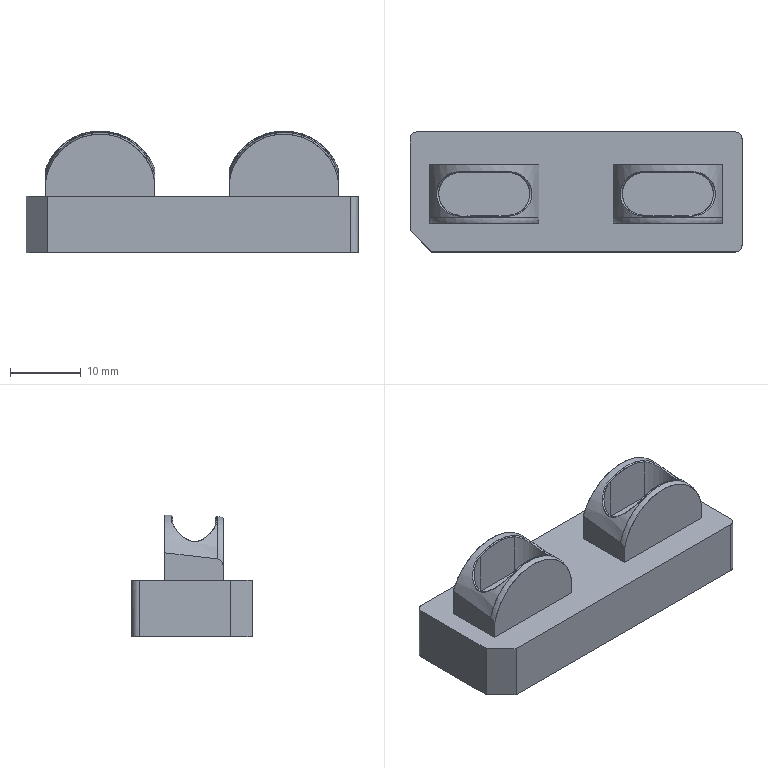NC program | PowerMill | posted with a generic post | part box 47 x 17 x 17.251 mm
Lines 18301 to 19119 of 158620:
N18398 M6
N18399 S8500 M03
N18400 G00 G90 X0.0 Y0.0
N18401 G43 Z9.8013 H3
N18402
N18403 G05 P10000 R8
N18404 X-25.6664 Y-17.9294
N18405 Z-8.25
N18406 G01 Z-9.45 F360.0
N18407 X-23.1365 Y-13.3007 F600.0
N18408 X-16.1394 Y-9.8021
N18409 X-20.3885
N18410 X-20.9549 Y-9.7974
N18411 G02 X-21.5212 Y-9.7435 I0.3338 J6.5029
N18412 G02 X-22.0876 Y-9.6275 I0.9782 J6.2202
N18413 G01 X-22.3708 Y-9.5453
N18414 G02 X-22.8859 Y-9.3503 I1.9528 J5.9372
N18415 G01 X-23.2203 Y-9.1901
N18416 X-23.5035 Y-9.0309
N18417 X-23.8008 Y-8.8385
N18418 X-24.1154 Y-8.6019
N18419 X-24.353 Y-8.3976
N18420 X-24.5418 Y-8.2169
N18421 X-24.7406 Y-8.0061
N18422 X-24.8895 Y-7.8308
N18423 X-25.0319 Y-7.6502
N18424 X-25.2306 Y-7.3669
N18425 X-25.4038 Y-7.0835
N18426 X-25.4857 Y-6.9339
N18427 X-25.5885 Y-6.7272
N18428 X-25.6837 Y-6.5169
N18429 X-25.794 Y-6.2335
N18430 X-25.8533 Y-6.0545
N18431 X-25.907 Y-5.8737
N18432 X-25.9622 Y-5.6668
N18433 X-26.0115 Y-5.4325
N18434 X-26.052 Y-5.1964
N18435 X-26.0938 Y-4.8168
N18436 X-26.1059 Y-4.5336
N18437 X-26.1081 Y3.6835
N18438 G02 X-26.0938 Y4.2501 I7.9765 J0.0813
N18439 G01 X-26.052 Y4.63
N18440 X-26.0216 Y4.8168
N18441 X-25.9622 Y5.1001
N18442 X-25.8867 Y5.3835
N18443 X-25.7943 Y5.6668
N18444 X-25.6837 Y5.9502
N18445 G02 X-25.4038 Y6.5169 I5.3267 J-2.2781
N18446 G01 X-25.2308 Y6.8002
N18447 X-25.0322 Y7.0835
N18448 X-24.9193 Y7.2288
N18449 X-24.7406 Y7.4395
N18450 X-24.5421 Y7.6502
N18451 X-24.353 Y7.8312
N18452 X-24.1157 Y8.0352
N18453 X-23.9528 Y8.1606
N18454 X-23.7866 Y8.2817
N18455 X-23.5035 Y8.4647
N18456 X-23.2203 Y8.6237
N18457 X-22.8868 Y8.7836
N18458 X-22.6539 Y8.8793
N18459 X-22.3708 Y8.9788
N18460 X-22.0876 Y9.0611
N18461 G02 X-21.5212 Y9.1771 I1.6038 J-6.3927
N18462 G02 X-20.9549 Y9.231 I0.8987 J-6.4341
N18463 G01 X-20.3885 Y9.2357
N18464 X-5.6635
N18465 X-5.0971 Y9.233
N18466 G02 X-4.5308 Y9.1845 I-0.264 J-6.4244
N18467 G02 X-3.9644 Y9.0744 I-0.9261 J-6.2735
N18468 G01 X-3.7406 Y9.0118
N18469 X-3.3981 Y8.899
N18470 X-3.1133 Y8.7836
N18471 X-2.8318 Y8.6505
N18472 X-2.5486 Y8.4955
N18473 X-2.2654 Y8.3174
N18474 X-2.1216 Y8.2169
N18475 X-1.9103 Y8.0562
N18476 X-1.699 Y7.878
N18477 X-1.4579 Y7.6502
N18478 G02 X-0.9679 Y7.0835 I-4.0616 J-4.0072
N18479 G01 X-0.8187 Y6.8709
N18480 G03 X0.8189 Y6.871 I0.8187 J0.5741
N18481 G01 X0.9679 Y7.0835
N18482 G02 X1.288 Y7.4714 I4.8718 J-3.6948
N18483 G01 X1.4579 Y7.6502
N18484 X1.699 Y7.878
N18485 X1.9103 Y8.0562
N18486 X2.0856 Y8.1898
N18487 X2.2654 Y8.3174
N18488 X2.5486 Y8.4955
N18489 X2.875 Y8.671
N18490 X3.1133 Y8.7836
N18491 X3.3981 Y8.899
N18492 X3.6813 Y8.9952
N18493 G02 X4.2476 Y9.1375 I1.8784 J-6.2784
N18494 G02 X4.814 Y9.2163 I1.1555 J-6.2283
N18495 G01 X5.0971 Y9.233
N18496 X5.6635 Y9.2357
N18497 X20.3885
N18498 X20.9549 Y9.231
N18499 G02 X21.5212 Y9.1771 I-0.3381 J-6.5471
N18500 G02 X22.0876 Y9.0611 I-1.0072 J-6.3617
N18501 G01 X22.2767 Y9.007
N18502 X22.6539 Y8.8793
N18503 X22.8868 Y8.7836
N18504 X23.2203 Y8.6237
N18505 X23.5035 Y8.4647
N18506 X23.6926 Y8.3433
N18507 X23.8784 Y8.2169
N18508 X24.1157 Y8.0352
N18509 X24.353 Y7.8312
N18510 X24.5421 Y7.6502
N18511 X24.7409 Y7.4395
N18512 X24.8896 Y7.2641
N18513 X25.0322 Y7.0836
N18514 X25.2308 Y6.8002
N18515 X25.3408 Y6.622
N18516 X25.4857 Y6.3677
N18517 X25.5903 Y6.159
N18518 X25.6662 Y5.9898
N18519 X25.7942 Y5.6668
N18520 X25.8867 Y5.3835
N18521 X25.9623 Y5.1002
N18522 X26.0216 Y4.8168
N18523 X26.052 Y4.63
N18524 X26.0938 Y4.2501
N18525 X26.1072 Y3.9668
N18526 Y-4.5335
N18527 X26.0938 Y-4.8168
N18528 X26.052 Y-5.1964
N18529 X26.0117 Y-5.4325
N18530 X25.9623 Y-5.6668
N18531 X25.8866 Y-5.9502
N18532 X25.7942 Y-6.2335
N18533 X25.6837 Y-6.5169
N18534 X25.5903 Y-6.7254
N18535 X25.4857 Y-6.9339
N18536 X25.4038 Y-7.0835
N18537 X25.2308 Y-7.3669
N18538 X25.0104 Y-7.6787
N18539 X24.9193 Y-7.7952
N18540 X24.7405 Y-8.0061
N18541 X24.5419 Y-8.2169
N18542 X24.353 Y-8.3976
N18543 X24.1154 Y-8.6019
N18544 X23.8163 Y-8.8277
N18545 X23.5035 Y-9.0309
N18546 X23.2203 Y-9.1901
N18547 X22.8859 Y-9.3503
N18548 X22.7006 Y-9.4269
N18549 X22.3708 Y-9.5453
N18550 G02 X21.8044 Y-9.6934 I-1.8826 J6.0394
N18551 G02 X21.2381 Y-9.7779 I-1.2236 J6.2663
N18552 G01 X20.9549 Y-9.7974
N18553 X20.3885 Y-9.8021
N18554 X5.6635
N18555 X5.0971 Y-9.7994
N18556 G02 X4.5308 Y-9.7509 I0.2749 J6.5522
N18557 G01 X4.3361 Y-9.7192
N18558 X3.9644 Y-9.6408
N18559 X3.6813 Y-9.5616
N18560 X3.3709 Y-9.4544
N18561 X3.1138 Y-9.3503
N18562 X2.8317 Y-9.2169
N18563 X2.5486 Y-9.0618
N18564 X2.2654 Y-8.8838
N18565 X2.0858 Y-8.7562
N18566 X1.9106 Y-8.6228
N18567 X1.699 Y-8.4444
N18568 X1.4582 Y-8.2169
N18569 X1.288 Y-8.0379
N18570 X1.101 Y-7.8187
N18571 X0.9679 Y-7.6502
N18572 X0.8189 Y-7.4377
N18573 G03 X-0.8187 Y-7.4375 I-0.8189 J-0.574
N18574 G01 X-0.9485 Y-7.6226
N18575 X-1.1327 Y-7.8589
N18576 X-1.2917 Y-8.0412
N18577 X-1.4582 Y-8.2169
N18578 X-1.7382 Y-8.4774
N18579 X-1.9106 Y-8.6228
N18580 X-2.0859 Y-8.7561
N18581 X-2.2654 Y-8.8838
N18582 X-2.5486 Y-9.0619
N18583 X-2.8317 Y-9.2169
N18584 X-3.1138 Y-9.3503
N18585 X-3.3981 Y-9.4654
N18586 X-3.6813 Y-9.5616
N18587 X-3.9644 Y-9.6408
N18588 X-4.1458 Y-9.6818
N18589 X-4.3282 Y-9.7172
N18590 X-4.5308 Y-9.7509
N18591 X-4.814 Y-9.7825
N18592 X-5.0971 Y-9.7994
N18593 X-5.6635 Y-9.8021
N18594 X-16.1394
N18595 G00 Z9.8013
N18596 G05 P0
N18597 (---------------)
N18598 ( END TOOLPATH : 精公基准台01-基准面偏置-D10 )
N18599 (---------------)
N18600 ( START TOOLPATH : 精公基准台01-外形侧光-D10 )
N18601 (---------------)
N18602 G00 X0.0 Y0.0 Z10.798
N18603 G05 P10000 R8
N18604 X-1.0177 Y-7.9884
N18605 Z-8.22
N18606 G01 Z-9.42 F360.0
N18607 G03 X-2.1184 Y-8.3147 I-0.1564 J-1.4919 F600.0
N18608 G02 X-5.2941 Y-9.432 I-3.1541 J3.8933
N18609 G01 X-12.9615 Y-9.4317
N18610 X-20.8143 Y-9.4313
N18611 G02 X-25.738 Y-4.3814 I0.0867 J5.0098
N18612 G01 Y3.8348
N18613 G02 X-20.8114 Y8.8649 I5.0101 J0.0207
N18614 G01 X-5.293 Y8.8656
N18615 G02 X-0.262 Y3.8337 I0.0208 J-5.0102
N18616 G01 Y-0.2846
N18617 Y-4.3822
N18618 G02 X-2.1184 Y-8.3147 I-5.0105 J-0.0392
N18619 G03 X-2.6659 Y-9.3238 I0.9443 J-1.1656
N18620 G01 X-1.0827 Y-7.9439
N18621 G03 X-2.1848 Y-8.2656 I-0.1627 J-1.4911
N18622 G02 X-5.2941 Y-9.352 I-3.0877 J3.8442
N18623 G01 X-12.9615
N18624 X-20.6289
N18625 G02 X-25.658 Y-4.3814 I-0.0957 J4.9326
N18626 G01 Y3.8337
N18627 G02 X-20.6289 Y8.7857 I4.933 J0.0198
N18628 G01 X-5.2941
N18629 G02 X-0.342 Y3.8337 I0.0219 J-4.9303
N18630 G01 Y-0.2846
N18631 Y-4.3814
N18632 G02 X-2.1848 Y-8.2656 I-4.9305 J-0.04
N18633 G03 X-2.7366 Y-9.2723 I0.9394 J-1.1694
N18634 G00 Z4.0618
N18635 G01 X24.9817 Y-7.9893 F10000.0
N18636 G00 Z-8.22
N18637 G01 Z-9.42 F360.0
N18638 G03 X23.8809 Y-8.3154 I-0.1568 J-1.4918 F600.0
N18639 G02 X20.8114 Y-9.4313 I-3.1532 J3.8939
N18640 G01 X5.293 Y-9.432
N18641 G02 X0.4219 Y-5.6778 I-0.0208 J5.0102
N18642 G02 X0.262 Y-4.3814 I4.8652 J1.2583
N18643 G01 Y-0.2846
N18644 Y3.8348
N18645 G02 X5.2941 Y8.8657 I5.0103 J0.0206
N18646 G01 X20.8143 Y8.8649
N18647 G02 X25.738 Y3.8337 I-0.0864 J-5.0095
N18648 G01 Y-4.3822
N18649 G02 X23.8809 Y-8.3154 I-5.0103 J-0.0393
N18650 G03 X23.3331 Y-9.3243 I0.944 J-1.1657
N18651 G01 X24.9156 Y-7.9449
N18652 G03 X23.8135 Y-8.2663 I-0.163 J-1.4911
N18653 G02 X20.6289 Y-9.352 I-3.0889 J3.8469
N18654 G01 X5.2941
N18655 G02 X0.4997 Y-5.6592 I-0.0219 J4.9302
N18656 G02 X0.342 Y-4.3814 I4.7864 J1.2396
N18657 G01 Y-0.2846
N18658 Y3.8337
N18659 G02 X5.2941 Y8.7857 I4.9302 J0.0217
N18660 G01 X20.6289
N18661 G02 X25.658 Y3.8337 I0.096 J-4.9322
N18662 G01 Y-4.3814
N18663 G02 X23.8135 Y-8.2663 I-4.9334 J-0.038
N18664 G03 X23.2615 Y-9.273 I0.9391 J-1.1697
N18665 G00 Z10.798
N18666 G05 P0
N18667 (---------------)
N18668 ( END TOOLPATH : 精公基准台01-外形侧光-D10 )
N18669 (---------------)
N18670 ( START TOOLPATH : 精公基准台01-基准台侧光-D10 )
N18671 (---------------)
N18672 G00 X0.0 Y0.0 Z9.8013
N18673 G05 P10000 R8
N18674 X28.7413 Y-16.6514
N18675 Z-16.15
N18676 G01 Z-17.35 F360.0
N18677 G03 X25.8898 Y-12.5442 I-1.4257 J2.0536 F600.0
N18678 G01 X25.8115 Y-12.5985
N18679 X25.8099 Y-12.5996
N18680 X25.8083 Y-12.6006
N18681 X25.6279 Y-12.7136
N18682 X25.6268 Y-12.7143
N18683 X25.6257 Y-12.715
N18684 X25.49 Y-12.7939
N18685 X25.4885 Y-12.7948
N18686 X25.487 Y-12.7956
N18687 X25.1708 Y-12.9619
N18688 X25.1693 Y-12.9627
N18689 X25.1677 Y-12.9635
N18690 X25.0174 Y-13.0343
N18691 X25.0164 Y-13.0348
N18692 X25.0153 Y-13.0353
N18693 X24.8494 Y-13.1077
N18694 X24.8478 Y-13.1084
N18695 X24.8462 Y-13.109
N18696 X24.5301 Y-13.231
N18697 X24.5278 Y-13.2319
N18698 X24.5254 Y-13.2326
N18699 X24.1404 Y-13.3544
N18700 X24.1384 Y-13.355
N18701 X24.1363 Y-13.3556
N18702 X23.8889 Y-13.4192
N18703 X23.887 Y-13.4197
N18704 X23.885 Y-13.4201
N18705 X23.5688 Y-13.4846
N18706 X23.5669 Y-13.485
N18707 X23.5649 Y-13.4853
N18708 X23.2488 Y-13.5337
N18709 X23.2465 Y-13.534
N18710 X23.2443 Y-13.5342
N18711 X22.9281 Y-13.5642
N18712 X22.9262 Y-13.5644
N18713 X22.9242 Y-13.5645
N18714 X22.608 Y-13.5788
N18715 X22.6064 Y-13.5789
N18716 X22.6047
N18717 X22.2885 Y-13.58
N18718 X22.2884
N18719 X22.2883
N18720 X-20.3914
N18721 X-20.3919
N18722 X-20.3925
N18723 X-20.7086 Y-13.5757
N18724 X-20.711 Y-13.5756
N18725 X-20.7134 Y-13.5755
N18726 X-21.0295 Y-13.5523
N18727 X-21.0321 Y-13.5521
N18728 X-21.0346 Y-13.5518
N18729 X-21.3507 Y-13.5082
N18730 X-21.3533 Y-13.5078
N18731 X-21.3558 Y-13.5074
N18732 X-21.672 Y-13.4429
N18733 X-21.6745 Y-13.4424
N18734 X-21.677 Y-13.4417
N18735 X-21.9932 Y-13.3556
N18736 X-21.9957 Y-13.3548
N18737 X-21.9982 Y-13.354
N18738 X-22.3144 Y-13.2449
N18739 X-22.3169 Y-13.244
N18740 X-22.3194 Y-13.243
N18741 X-22.6356 Y-13.1093
N18742 X-22.6375 Y-13.1084
N18743 X-22.6393 Y-13.1076
N18744 X-22.7912 Y-13.034
N18745 X-22.7924 Y-13.0333
N18746 X-22.7937 Y-13.0327
N18747 X-22.958 Y-12.9458
N18748 X-22.9599 Y-12.9447
N18749 X-22.9618 Y-12.9436
N18750 X-23.278 Y-12.7531
N18751 X-23.2806 Y-12.7515
N18752 X-23.2831 Y-12.7498
N18753 X-23.5992 Y-12.525
N18754 X-23.6011 Y-12.5236
N18755 X-23.603 Y-12.5221
N18756 X-23.7647 Y-12.392
N18757 X-23.766 Y-12.391
N18758 X-23.7673 Y-12.3899
N18759 X-23.9217 Y-12.2548
N18760 X-23.9231 Y-12.2535
N18761 X-23.9244 Y-12.2523
N18762 X-24.113 Y-12.0712
N18763 X-24.1135 Y-12.0707
N18764 X-24.1141 Y-12.0701
N18765 X-27.087 Y-9.0972
N18766 X-27.0877 Y-9.0965
N18767 X-27.0884 Y-9.0958
N18768 X-27.2679 Y-8.9072
N18769 X-27.2692 Y-8.9059
N18770 X-27.2704 Y-8.9045
N18771 X-27.4071 Y-8.7467
N18772 X-27.4081 Y-8.7454
N18773 X-27.4092 Y-8.7442
N18774 X-27.5354 Y-8.5858
N18775 X-27.5367 Y-8.5841
N18776 X-27.5379 Y-8.5824
N18777 X-27.7279 Y-8.3162
N18778 X-27.7296 Y-8.3137
N18779 X-27.7312 Y-8.3112
N18780 X-27.9528 Y-7.9451
N18781 X-27.9541 Y-7.9429
N18782 X-27.9553 Y-7.9407
N18783 X-28.0498 Y-7.7595
N18784 X-28.0505 Y-7.7583
N18785 X-28.0511 Y-7.757
N18786 X-28.1156 Y-7.622
N18787 X-28.1164 Y-7.6202
N18788 X-28.1172 Y-7.6184
N18789 X-28.2495 Y-7.3022
N18790 X-28.2505 Y-7.2997
N18791 X-28.2514 Y-7.2972
N18792 X-28.3593 Y-6.981
N18793 X-28.3601 Y-6.9785
N18794 X-28.3608 Y-6.976
N18795 X-28.4458 Y-6.6598
N18796 X-28.4464 Y-6.6573
N18797 X-28.447 Y-6.6548
N18798 X-28.5103 Y-6.3386
N18799 X-28.5107 Y-6.3361
N18800 X-28.5111 Y-6.3336
N18801 X-28.5535 Y-6.0174
N18802 X-28.5538 Y-6.0149
N18803 X-28.5541 Y-6.0124
N18804 X-28.5762 Y-5.6962
N18805 X-28.5763 Y-5.6939
N18806 X-28.5764 Y-5.6915
N18807 X-28.58 Y-5.3754
N18808 Y-5.3749
N18809 Y-5.3745
N18810 X-28.5792 Y7.5875
N18811 Y7.5891
N18812 Y7.5907
N18813 X-28.5663 Y7.9069
N18814 X-28.5662 Y7.909
N18815 X-28.5661 Y7.9111
N18816 X-28.5363 Y8.2273
N18817 X-28.536 Y8.2294
N18818 X-28.5358 Y8.2315
N18819 X-28.489 Y8.5476
N18820 X-28.4887 Y8.5498
N18821 X-28.4883 Y8.5519
N18822 X-28.424 Y8.868
N18823 X-28.4236 Y8.8701
N18824 X-28.423 Y8.8722
N18825 X-28.3407 Y9.1884
N18826 X-28.3402 Y9.1905
N18827 X-28.3395 Y9.1926
N18828 X-28.2384 Y9.5087
N18829 X-28.2377 Y9.5108
N18830 X-28.2369 Y9.5129
N18831 X-28.1162 Y9.8291
N18832 X-28.1156 Y9.8306
N18833 X-28.1149 Y9.8322
N18834 X-28.0524 Y9.9774
N18835 X-28.0519 Y9.9785
N18836 X-28.0514 Y9.9796
N18837 X-27.9717 Y10.1505
N18838 X-27.9709 Y10.1521
N18839 X-27.9701 Y10.1537
N18840 X-27.8052 Y10.4698
N18841 X-27.8044 Y10.4713
N18842 X-27.8036 Y10.4727
N18843 X-27.7321 Y10.5969
N18844 X-27.7314 Y10.598
N18845 X-27.7308 Y10.5991
N18846 X-27.6121 Y10.791
N18847 X-27.6111 Y10.7926
N18848 X-27.61 Y10.7942
N18849 X-27.4126 Y11.0822
N18850 X-27.4111 Y11.0844
N18851 X-27.4095 Y11.0865
N18852 X-27.1384 Y11.4307
N18853 X-27.1366 Y11.433
N18854 X-27.1347 Y11.4351
N18855 X-26.8465 Y11.7513
N18856 X-26.8453 Y11.7526
N18857 X-26.844 Y11.7538
N18858 X-26.771 Y11.8272
N18859 X-26.7699 Y11.8283
N18860 X-26.7688 Y11.8293
N18861 X-26.5075 Y12.0721
N18862 X-26.5055 Y12.074
N18863 X-26.5033 Y12.0758
N18864 X-26.1323 Y12.3756
N18865 X-26.13 Y12.3774
N18866 X-26.1276 Y12.3791
N18867 X-25.8115 Y12.5985
N18868 X-25.8099 Y12.5996
N18869 X-25.8083 Y12.6006
N18870 X-25.6279 Y12.7136
N18871 X-25.6268 Y12.7143
N18872 X-25.6257 Y12.715
N18873 X-25.49 Y12.7939
N18874 X-25.4885 Y12.7948
N18875 X-25.487 Y12.7956
N18876 X-25.1708 Y12.9619
N18877 X-25.1693 Y12.9627
N18878 X-25.1677 Y12.9635
N18879 X-25.0174 Y13.0343
N18880 X-25.0164 Y13.0348
N18881 X-25.0153 Y13.0353
N18882 X-24.8494 Y13.1077
N18883 X-24.8478 Y13.1084
N18884 X-24.8462 Y13.109
N18885 X-24.5301 Y13.231
N18886 X-24.528 Y13.2318
N18887 X-24.5259 Y13.2325
N18888 X-24.2097 Y13.3346
N18889 X-24.2076 Y13.3353
N18890 X-24.2055 Y13.3359
N18891 X-23.8894 Y13.4191
N18892 X-23.8872 Y13.4196
N18893 X-23.885 Y13.4201
N18894 X-23.5688 Y13.4846
N18895 X-23.5669 Y13.485
N18896 X-23.5649 Y13.4853
N18897 X-23.2488 Y13.5337
N18898 X-23.2465 Y13.534
N18899 X-23.2443 Y13.5342
N18900 X-22.9281 Y13.5642
N18901 X-22.9262 Y13.5644
N18902 X-22.9242 Y13.5645
N18903 X-22.608 Y13.5788
N18904 X-22.6064 Y13.5789
N18905 X-22.6047
N18906 X-22.2885 Y13.58
N18907 X-22.2884
N18908 X-22.2883
N18909 X0.0
N18910 X22.2883
N18911 X22.2884
N18912 X22.2885
N18913 X22.6047 Y13.5789
N18914 X22.6063
N18915 X22.6079 Y13.5788
N18916 X22.924 Y13.5652
N18917 X22.9262 Y13.565
N18918 X22.9283 Y13.5649
N18919 X23.2444 Y13.5342
N18920 X23.2465 Y13.534
N18921 X23.2486 Y13.5337
N18922 X23.5648 Y13.486
N18923 X23.5669 Y13.4857
N18924 X23.569 Y13.4853
N18925 X23.8852 Y13.4201
N18926 X23.887 Y13.4197
N18927 X23.8889 Y13.4192
N18928 X24.1362 Y13.3556
N18929 X24.1384 Y13.355
N18930 X24.1405 Y13.3544
N18931 X24.5254 Y13.2324
N18932 X24.5278 Y13.2317
N18933 X24.53 Y13.2308
N18934 X24.8462 Y13.109
N18935 X24.8478 Y13.1084
N18936 X24.8495 Y13.1077
N18937 X25.0153 Y13.0353
N18938 X25.0164 Y13.0348
N18939 X25.0175 Y13.0343
N18940 X25.1678 Y12.9632
N18941 X25.1693 Y12.9624
N18942 X25.1708 Y12.9617
N18943 X25.4869 Y12.7956
N18944 X25.4885 Y12.7948
N18945 X25.49 Y12.7939
N18946 X25.6257 Y12.715
N18947 X25.6267 Y12.7143
N18948 X25.6278 Y12.7137
N18949 X25.8082 Y12.601
N18950 X25.8098 Y12.6
N18951 X25.8114 Y12.599
N18952 X26.1055 Y12.3955
N18953 X26.1077 Y12.3939
N18954 X26.1098 Y12.3923
N18955 X26.4479 Y12.1238
N18956 X26.4501 Y12.1219
N18957 X26.4523 Y12.12
N18958 X26.7684 Y11.8297
N18959 X26.7697 Y11.8284
N18960 X26.771 Y11.8272
N18961 X26.844 Y11.7538
N18962 X26.8451 Y11.7527
N18963 X26.8462 Y11.7516
N18964 X27.0893 Y11.4878
N18965 X27.0911 Y11.4857
N18966 X27.0929 Y11.4836
N18967 X27.3883 Y11.1152
N18968 X27.3901 Y11.1129
N18969 X27.3918 Y11.1105
N18970 X27.6098 Y10.7944
N18971 X27.6108 Y10.7927
N18972 X27.6119 Y10.7911
N18973 X27.7308 Y10.5991
N18974 X27.7314 Y10.598
N18975 X27.7321 Y10.5969
N18976 X27.8036 Y10.4727
N18977 X27.8044 Y10.4713
N18978 X27.8052 Y10.4698
N18979 X27.9703 Y10.1537
N18980 X27.9713 Y10.1516
N18981 X27.9723 Y10.1495
N18982 X28.1144 Y9.8333
N18983 X28.1153 Y9.8312
N18984 X28.1162 Y9.8291
N18985 X28.237 Y9.5129
N18986 X28.2378 Y9.5108
N18987 X28.2385 Y9.5087
N18988 X28.3396 Y9.1926
N18989 X28.3402 Y9.1905
N18990 X28.3408 Y9.1884
N18991 X28.4231 Y8.8722
N18992 X28.4236 Y8.87
N18993 X28.4241 Y8.8678
N18994 X28.4876 Y8.5517
N18995 X28.488 Y8.5498
N18996 X28.4883 Y8.5478
N18997 X28.5357 Y8.2317
N18998 X28.536 Y8.2294
N18999 X28.5363 Y8.2271
N19000 X28.5653 Y7.911
N19001 X28.5655 Y7.909
N19002 X28.5656 Y7.9071
N19003 X28.5792 Y7.5909
N19004 Y7.5892
N19005 Y7.5875
N19006 Y-7.5875
N19007 Y-7.5891
N19008 Y-7.5907
N19009 X28.5663 Y-7.9069
N19010 X28.5662 Y-7.909
N19011 X28.5661 Y-7.9112
N19012 X28.5363 Y-8.2273
N19013 X28.536 Y-8.2294
N19014 X28.5357 Y-8.2315
N19015 X28.489 Y-8.5476
N19016 X28.4887 Y-8.5498
N19017 X28.4883 Y-8.5519
N19018 X28.424 Y-8.868
N19019 X28.4236 Y-8.8701
N19020 X28.4231 Y-8.8722
N19021 X28.3407 Y-9.1884
N19022 X28.3402 Y-9.1905
N19023 X28.3395 Y-9.1926
N19024 X28.2384 Y-9.5087
N19025 X28.2377 Y-9.5108
N19026 X28.2369 Y-9.5129
N19027 X28.1162 Y-9.8291
N19028 X28.1156 Y-9.8306
N19029 X28.1149 Y-9.8322
N19030 X28.0524 Y-9.9774
N19031 X28.0519 Y-9.9785
N19032 X28.0514 Y-9.9796
N19033 X27.9717 Y-10.1505
N19034 X27.9709 Y-10.1521
N19035 X27.9701 Y-10.1537
N19036 X27.8052 Y-10.4698
N19037 X27.8044 Y-10.4713
N19038 X27.8036 Y-10.4727
N19039 X27.7321 Y-10.5969
N19040 X27.7314 Y-10.598
N19041 X27.7308 Y-10.5991
N19042 X27.6121 Y-10.791
N19043 X27.6111 Y-10.7926
N19044 X27.61 Y-10.7942
N19045 X27.4126 Y-11.0822
N19046 X27.4111 Y-11.0844
N19047 X27.4095 Y-11.0865
N19048 X27.1384 Y-11.4307
N19049 X27.1366 Y-11.433
N19050 X27.1347 Y-11.4351
N19051 X26.8465 Y-11.7513
N19052 X26.8453 Y-11.7526
N19053 X26.844 Y-11.7538
N19054 X26.771 Y-11.8272
N19055 X26.7699 Y-11.8283
N19056 X26.7688 Y-11.8293
N19057 X26.5075 Y-12.0721
N19058 X26.5055 Y-12.074
N19059 X26.5033 Y-12.0758
N19060 X26.1323 Y-12.3756
N19061 X26.13 Y-12.3774
N19062 X26.1276 Y-12.3791
N19063 X25.8898 Y-12.5442
N19064 G03 X28.7413 Y-16.6514 I1.4258 J-2.0536
N19065 G01 X28.6905 Y-16.5892
N19066 G03 X25.839 Y-12.482 I-1.4257 J2.0536
N19067 G01 X25.7659 Y-12.5328
N19068 X25.5854 Y-12.6458
N19069 X25.4497 Y-12.7248
N19070 X25.1336 Y-12.8911
N19071 X24.9833 Y-12.962
N19072 X24.8174 Y-13.0344
N19073 X24.5013 Y-13.1564
N19074 X24.1163 Y-13.2781
N19075 X23.869 Y-13.3417
N19076 X23.5529 Y-13.4062
N19077 X23.2367 Y-13.4546
N19078 X22.9206 Y-13.4846
N19079 X22.6044 Y-13.4989
N19080 X22.2883 Y-13.5
N19081 X-20.3914
N19082 X-20.7075 Y-13.4957
N19083 X-21.0237 Y-13.4725
N19084 X-21.3398 Y-13.429
N19085 X-21.656 Y-13.3645
N19086 X-21.9721 Y-13.2784
N19087 X-22.2883 Y-13.1693
N19088 X-22.6044 Y-13.0356
N19089 X-22.7563 Y-12.962
N19090 X-22.9206 Y-12.875
N19091 X-23.2367 Y-12.6846
N19092 X-23.5529 Y-12.4598
N19093 X-23.7146 Y-12.3297
N19094 X-23.869 Y-12.1946
N19095 X-24.0575 Y-12.0135
N19096 X-27.0305 Y-9.0406
N19097 X-27.2099 Y-8.8521
N19098 X-27.3466 Y-8.6943
N19099 X-27.4728 Y-8.5359
N19100 X-27.6627 Y-8.2698
N19101 X-27.8844 Y-7.9036
N19102 X-27.9789 Y-7.7225
N19103 X-28.0434 Y-7.5875
N19104 X-28.1757 Y-7.2714
N19105 X-28.2836 Y-6.9552
N19106 X-28.3685 Y-6.6391
N19107 X-28.4318 Y-6.3229
N19108 X-28.4743 Y-6.0068
N19109 X-28.4964 Y-5.6906
N19110 X-28.5 Y-5.3745
N19111 Y7.2714
N19112 X-28.4992 Y7.5875
N19113 X-28.4864 Y7.9036
N19114 X-28.4566 Y8.2198
N19115 X-28.4099 Y8.5359
N19116 X-28.3456 Y8.8521
N19117 X-28.2633 Y9.1682
N19118 X-28.1622 Y9.4844
N19119 X-28.0415 Y9.8005
N19120 X-27.9789 Y9.9458
N19121 X-27.8992 Y10.1167
N19122 X-27.7343 Y10.4328
N19123 X-27.6627 Y10.557
N19124 X-27.544 Y10.749
N19125 X-27.3466 Y11.037
N19126 X-27.0756 Y11.3812
N19127 X-26.7873 Y11.6974
N19128 X-26.7143 Y11.7707
N19129 X-26.4531 Y12.0135
N19130 X-26.082 Y12.3133
N19131 X-25.7659 Y12.5328
N19132 X-25.5854 Y12.6458
N19133 X-25.4497 Y12.7248
N19134 X-25.1336 Y12.8911
N19135 X-24.9833 Y12.962
N19136 X-24.8174 Y13.0344
N19137 X-24.5013 Y13.1564
N19138 X-24.1851 Y13.2585
N19139 X-23.869 Y13.3417
N19140 X-23.5529 Y13.4062
N19141 X-23.2367 Y13.4546
N19142 X-22.9206 Y13.4846
N19143 X-22.6044 Y13.4989
N19144 X-22.2883 Y13.5
N19145 X0.0
N19146 X22.2883
N19147 X22.6044 Y13.4989
N19148 X22.9206 Y13.4852
N19149 X23.2367 Y13.4546
N19150 X23.5529 Y13.4069
N19151 X23.869 Y13.3417
N19152 X24.1163 Y13.2781
N19153 X24.5013 Y13.1562
N19154 X24.8174 Y13.0344
N19155 X24.9832 Y12.962
N19156 X25.1336 Y12.8909
N19157 X25.4497 Y12.7248
N19158 X25.5854 Y12.6458
N19159 X25.7659 Y12.5332
N19160 X26.06 Y12.3297
N19161 X26.3982 Y12.0611
N19162 X26.7143 Y11.7707
N19163 X26.7873 Y11.6974
N19164 X27.0305 Y11.4335
N19165 X27.3259 Y11.0651
N19166 X27.5439 Y10.749
N19167 X27.6627 Y10.557
N19168 X27.7343 Y10.4328
N19169 X27.8993 Y10.1167
N19170 X28.0415 Y9.8005
N19171 X28.1623 Y9.4844
N19172 X28.2634 Y9.1682
N19173 X28.3457 Y8.8521
N19174 X28.4092 Y8.5359
N19175 X28.4566 Y8.2198
N19176 X28.4856 Y7.9036
N19177 X28.4992 Y7.5875
N19178 X28.5 Y7.2714
N19179 Y-7.2714
N19180 X28.4992 Y-7.5875
N19181 X28.4864 Y-7.9036
N19182 X28.4566 Y-8.2198
N19183 X28.4099 Y-8.5359
N19184 X28.3456 Y-8.8521
N19185 X28.2633 Y-9.1682
N19186 X28.1622 Y-9.4844
N19187 X28.0415 Y-9.8005
N19188 X27.9789 Y-9.9458
N19189 X27.8992 Y-10.1167
N19190 X27.7343 Y-10.4328
N19191 X27.6627 Y-10.557
N19192 X27.544 Y-10.749
N19193 X27.3466 Y-11.037
N19194 X27.0756 Y-11.3812
N19195 X26.7873 Y-11.6974
N19196 X26.7143 Y-11.7707
N19197 X26.4531 Y-12.0135
N19198 X26.082 Y-12.3133
N19199 X25.839 Y-12.482
N19200 G03 X28.6905 Y-16.5893 I1.4258 J-2.0537
N19201 G00 Z9.8013
N19202 G05 P0
N19203 (---------------)
N19204 ( END TOOLPATH : 精公基准台01-基准台侧光-D10 )
N19205 (---------------)
N19206
N19207 M05
N19208 G53 Z0.0
N19209 (---------------)
N19210 ( START TOOLPATH : 精公精光01-平行-R1.5 )
N19211 (---------------)
N19212 ( TOOL NO.    :22 )
N19213 ( TOOL TYPE   : BALLNOSED)
N19214 ( TOOL ID     : R1.5_1_1)
N19215 ( TOOL DIA    : 3.0 LENGTH 63.12)
N19216 T22